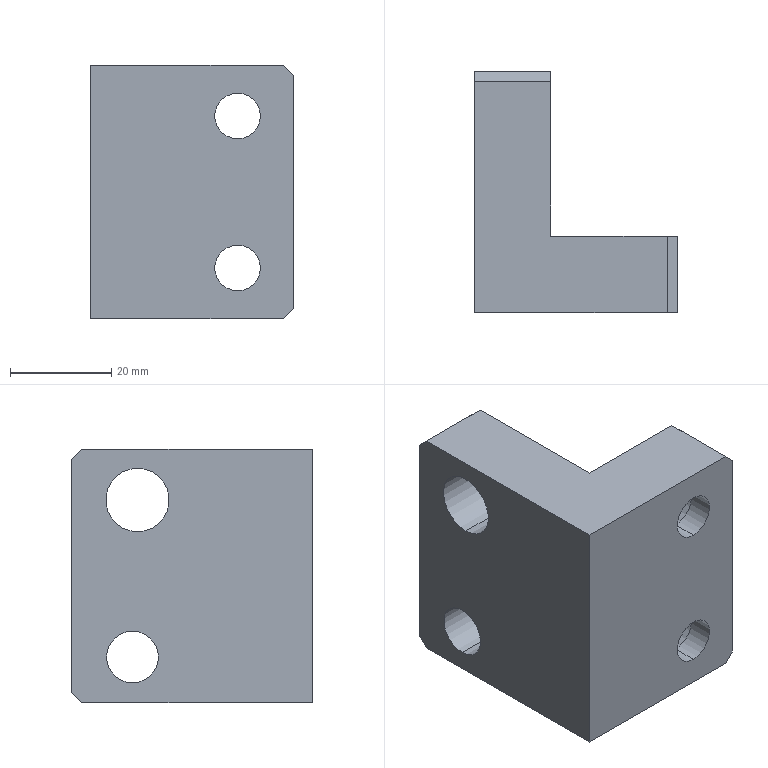Part | SolidWorks | features HoleWzd 3, Chamfer 1, Extrusion 1 | 1 solid | 26 faces | box 40 x 47.5 x 50 mm | volume 47018 mm3 | plane 14 | cylinder 12 | commonest cylinder face diameters 9 x4 15 x4 10.2 x2 12.5 x2
STEP:
#1=CARTESIAN_POINT('',(-40.82,7.906,14.1));
#2=VERTEX_POINT('',#1);
#3=CARTESIAN_POINT('',(-40.82,7.906,3.9));
#4=VERTEX_POINT('',#3);
#5=CARTESIAN_POINT('',(-40.82,7.906,9.));
#6=DIRECTION('',(1.,0.,0.));
#7=DIRECTION('',(0.,0.,-1.));
#8=AXIS2_PLACEMENT_3D('',#5,#6,#7);
#9=CIRCLE('',#8,5.1);
#10=EDGE_CURVE('',#2,#4,#9,.T.);
#11=ORIENTED_EDGE('',*,*,#10,.F.);
#12=CARTESIAN_POINT('',(-25.82,7.906,14.1));
#13=VERTEX_POINT('',#12);
#14=CARTESIAN_POINT('',(-25.82,7.906,14.1));
#15=DIRECTION('',(1.,0.,0.));
#16=VECTOR('',#15,1000.);
#17=LINE('',#14,#16);
#18=EDGE_CURVE('',#2,#13,#17,.T.);
#19=ORIENTED_EDGE('',*,*,#18,.T.);
#20=CARTESIAN_POINT('',(-25.82,7.906,3.9));
#21=VERTEX_POINT('',#20);
#22=CARTESIAN_POINT('',(-25.82,7.906,9.));
#23=DIRECTION('',(1.,0.,0.));
#24=DIRECTION('',(0.,0.,-1.));
#25=AXIS2_PLACEMENT_3D('',#22,#23,#24);
#26=CIRCLE('',#25,5.1);
#27=EDGE_CURVE('',#13,#21,#26,.T.);
#28=ORIENTED_EDGE('',*,*,#27,.T.);
#29=CARTESIAN_POINT('',(-25.82,7.906,3.9));
#30=DIRECTION('',(1.,0.,0.));
#31=VECTOR('',#30,1000.);
#32=LINE('',#29,#31);
#33=EDGE_CURVE('',#4,#21,#32,.T.);
#34=ORIENTED_EDGE('',*,*,#33,.F.);
#35=EDGE_LOOP('',(#11,#19,#28,#34));
#36=FACE_OUTER_BOUND('',#35,.T.);
#37=CARTESIAN_POINT('',(-25.82,7.906,9.));
#38=DIRECTION('',(1.,0.,0.));
#39=DIRECTION('',(0.,0.,-1.));
#40=AXIS2_PLACEMENT_3D('',#37,#38,#39);
#41=CYLINDRICAL_SURFACE('',#40,5.1);
#42=ADVANCED_FACE('',(#36),#41,.F.);
#43=CARTESIAN_POINT('',(-40.82,6.906,46.25));
#44=VERTEX_POINT('',#43);
#45=CARTESIAN_POINT('',(-40.82,6.906,33.75));
#46=VERTEX_POINT('',#45);
#47=CARTESIAN_POINT('',(-40.82,6.906,40.));
#48=DIRECTION('',(1.,0.,0.));
#49=DIRECTION('',(0.,0.,-1.));
#50=AXIS2_PLACEMENT_3D('',#47,#48,#49);
#51=CIRCLE('',#50,6.25);
#52=EDGE_CURVE('',#44,#46,#51,.T.);
#53=ORIENTED_EDGE('',*,*,#52,.F.);
#54=CARTESIAN_POINT('',(-25.82,6.906,46.25));
#55=VERTEX_POINT('',#54);
#56=CARTESIAN_POINT('',(-25.82,6.906,46.25));
#57=DIRECTION('',(1.,0.,0.));
#58=VECTOR('',#57,1000.);
#59=LINE('',#56,#58);
#60=EDGE_CURVE('',#44,#55,#59,.T.);
#61=ORIENTED_EDGE('',*,*,#60,.T.);
#62=CARTESIAN_POINT('',(-25.82,6.906,33.75));
#63=VERTEX_POINT('',#62);
#64=CARTESIAN_POINT('',(-25.82,6.906,40.));
#65=DIRECTION('',(1.,0.,0.));
#66=DIRECTION('',(0.,0.,-1.));
#67=AXIS2_PLACEMENT_3D('',#64,#65,#66);
#68=CIRCLE('',#67,6.25);
#69=EDGE_CURVE('',#55,#63,#68,.T.);
#70=ORIENTED_EDGE('',*,*,#69,.T.);
#71=CARTESIAN_POINT('',(-25.82,6.906,33.75));
#72=DIRECTION('',(1.,0.,0.));
#73=VECTOR('',#72,1000.);
#74=LINE('',#71,#73);
#75=EDGE_CURVE('',#46,#63,#74,.T.);
#76=ORIENTED_EDGE('',*,*,#75,.F.);
#77=EDGE_LOOP('',(#53,#61,#70,#76));
#78=FACE_OUTER_BOUND('',#77,.T.);
#79=CARTESIAN_POINT('',(-25.82,6.906,40.));
#80=DIRECTION('',(1.,0.,0.));
#81=DIRECTION('',(0.,0.,-1.));
#82=AXIS2_PLACEMENT_3D('',#79,#80,#81);
#83=CYLINDRICAL_SURFACE('',#82,6.25);
#84=ADVANCED_FACE('',(#78),#83,.F.);
#85=CARTESIAN_POINT('',(-11.82,-22.594,2.5));
#86=VERTEX_POINT('',#85);
#87=CARTESIAN_POINT('',(-11.82,-22.594,17.5));
#88=VERTEX_POINT('',#87);
#89=CARTESIAN_POINT('',(-11.82,-22.594,10.));
#90=DIRECTION('',(0.,1.,0.));
#91=DIRECTION('',(0.,0.,1.));
#92=AXIS2_PLACEMENT_3D('',#89,#90,#91);
#93=CIRCLE('',#92,7.5);
#94=EDGE_CURVE('',#86,#88,#93,.T.);
#95=ORIENTED_EDGE('',*,*,#94,.F.);
#96=CARTESIAN_POINT('',(-11.82,-12.594,2.5));
#97=VERTEX_POINT('',#96);
#98=CARTESIAN_POINT('',(-11.82,-12.594,2.5));
#99=DIRECTION('',(0.,1.,0.));
#100=VECTOR('',#99,1000.);
#101=LINE('',#98,#100);
#102=EDGE_CURVE('',#86,#97,#101,.T.);
#103=ORIENTED_EDGE('',*,*,#102,.T.);
#104=CARTESIAN_POINT('',(-11.82,-12.594,17.5));
#105=VERTEX_POINT('',#104);
#106=CARTESIAN_POINT('',(-11.82,-12.594,10.));
#107=DIRECTION('',(0.,1.,0.));
#108=DIRECTION('',(0.,0.,1.));
#109=AXIS2_PLACEMENT_3D('',#106,#107,#108);
#110=CIRCLE('',#109,7.5);
#111=EDGE_CURVE('',#97,#105,#110,.T.);
#112=ORIENTED_EDGE('',*,*,#111,.T.);
#113=CARTESIAN_POINT('',(-11.82,-12.594,17.5));
#114=DIRECTION('',(0.,1.,0.));
#115=VECTOR('',#114,1000.);
#116=LINE('',#113,#115);
#117=EDGE_CURVE('',#88,#105,#116,.T.);
#118=ORIENTED_EDGE('',*,*,#117,.F.);
#119=EDGE_LOOP('',(#95,#103,#112,#118));
#120=FACE_OUTER_BOUND('',#119,.T.);
#121=CARTESIAN_POINT('',(-11.82,-12.594,10.));
#122=DIRECTION('',(0.,1.,0.));
#123=DIRECTION('',(0.,0.,1.));
#124=AXIS2_PLACEMENT_3D('',#121,#122,#123);
#125=CYLINDRICAL_SURFACE('',#124,7.5);
#126=ADVANCED_FACE('',(#120),#125,.F.);
#127=CARTESIAN_POINT('',(-11.82,-27.594,5.5));
#128=VERTEX_POINT('',#127);
#129=CARTESIAN_POINT('',(-11.82,-27.594,14.5));
#130=VERTEX_POINT('',#129);
#131=CARTESIAN_POINT('',(-11.82,-27.594,10.));
#132=DIRECTION('',(0.,1.,0.));
#133=DIRECTION('',(0.,0.,1.));
#134=AXIS2_PLACEMENT_3D('',#131,#132,#133);
#135=CIRCLE('',#134,4.5);
#136=EDGE_CURVE('',#128,#130,#135,.T.);
#137=ORIENTED_EDGE('',*,*,#136,.F.);
#138=CARTESIAN_POINT('',(-11.82,-22.594,5.5));
#139=VERTEX_POINT('',#138);
#140=CARTESIAN_POINT('',(-11.82,-12.594,5.5));
#141=DIRECTION('',(0.,1.,0.));
#142=VECTOR('',#141,1000.);
#143=LINE('',#140,#142);
#144=EDGE_CURVE('',#128,#139,#143,.T.);
#145=ORIENTED_EDGE('',*,*,#144,.T.);
#146=CARTESIAN_POINT('',(-11.82,-22.594,14.5));
#147=VERTEX_POINT('',#146);
#148=CARTESIAN_POINT('',(-11.82,-22.594,10.));
#149=DIRECTION('',(0.,1.,0.));
#150=DIRECTION('',(0.,0.,1.));
#151=AXIS2_PLACEMENT_3D('',#148,#149,#150);
#152=CIRCLE('',#151,4.5);
#153=EDGE_CURVE('',#139,#147,#152,.T.);
#154=ORIENTED_EDGE('',*,*,#153,.T.);
#155=CARTESIAN_POINT('',(-11.82,-12.594,14.5));
#156=DIRECTION('',(0.,1.,0.));
#157=VECTOR('',#156,1000.);
#158=LINE('',#155,#157);
#159=EDGE_CURVE('',#130,#147,#158,.T.);
#160=ORIENTED_EDGE('',*,*,#159,.F.);
#161=EDGE_LOOP('',(#137,#145,#154,#160));
#162=FACE_OUTER_BOUND('',#161,.T.);
#163=CARTESIAN_POINT('',(-11.82,-12.594,10.));
#164=DIRECTION('',(0.,1.,0.));
#165=DIRECTION('',(0.,0.,1.));
#166=AXIS2_PLACEMENT_3D('',#163,#164,#165);
#167=CYLINDRICAL_SURFACE('',#166,4.5);
#168=ADVANCED_FACE('',(#162),#167,.F.);
#169=CARTESIAN_POINT('',(-11.82,-22.594,32.5));
#170=VERTEX_POINT('',#169);
#171=CARTESIAN_POINT('',(-11.82,-22.594,47.5));
#172=VERTEX_POINT('',#171);
#173=CARTESIAN_POINT('',(-11.82,-22.594,40.));
#174=DIRECTION('',(0.,1.,0.));
#175=DIRECTION('',(0.,0.,1.));
#176=AXIS2_PLACEMENT_3D('',#173,#174,#175);
#177=CIRCLE('',#176,7.5);
#178=EDGE_CURVE('',#170,#172,#177,.T.);
#179=ORIENTED_EDGE('',*,*,#178,.F.);
#180=CARTESIAN_POINT('',(-11.82,-12.594,32.5));
#181=VERTEX_POINT('',#180);
#182=CARTESIAN_POINT('',(-11.82,-12.594,32.5));
#183=DIRECTION('',(0.,1.,0.));
#184=VECTOR('',#183,1000.);
#185=LINE('',#182,#184);
#186=EDGE_CURVE('',#170,#181,#185,.T.);
#187=ORIENTED_EDGE('',*,*,#186,.T.);
#188=CARTESIAN_POINT('',(-11.82,-12.594,47.5));
#189=VERTEX_POINT('',#188);
#190=CARTESIAN_POINT('',(-11.82,-12.594,40.));
#191=DIRECTION('',(0.,1.,0.));
#192=DIRECTION('',(0.,0.,1.));
#193=AXIS2_PLACEMENT_3D('',#190,#191,#192);
#194=CIRCLE('',#193,7.5);
#195=EDGE_CURVE('',#181,#189,#194,.T.);
#196=ORIENTED_EDGE('',*,*,#195,.T.);
#197=CARTESIAN_POINT('',(-11.82,-12.594,47.5));
#198=DIRECTION('',(0.,1.,0.));
#199=VECTOR('',#198,1000.);
#200=LINE('',#197,#199);
#201=EDGE_CURVE('',#172,#189,#200,.T.);
#202=ORIENTED_EDGE('',*,*,#201,.F.);
#203=EDGE_LOOP('',(#179,#187,#196,#202));
#204=FACE_OUTER_BOUND('',#203,.T.);
#205=CARTESIAN_POINT('',(-11.82,-12.594,40.));
#206=DIRECTION('',(0.,1.,0.));
#207=DIRECTION('',(0.,0.,1.));
#208=AXIS2_PLACEMENT_3D('',#205,#206,#207);
#209=CYLINDRICAL_SURFACE('',#208,7.5);
#210=ADVANCED_FACE('',(#204),#209,.F.);
#211=CARTESIAN_POINT('',(-11.82,-27.594,35.5));
#212=VERTEX_POINT('',#211);
#213=CARTESIAN_POINT('',(-11.82,-27.594,44.5));
#214=VERTEX_POINT('',#213);
#215=CARTESIAN_POINT('',(-11.82,-27.594,40.));
#216=DIRECTION('',(0.,1.,0.));
#217=DIRECTION('',(0.,0.,1.));
#218=AXIS2_PLACEMENT_3D('',#215,#216,#217);
#219=CIRCLE('',#218,4.5);
#220=EDGE_CURVE('',#212,#214,#219,.T.);
#221=ORIENTED_EDGE('',*,*,#220,.F.);
#222=CARTESIAN_POINT('',(-11.82,-22.594,35.5));
#223=VERTEX_POINT('',#222);
#224=CARTESIAN_POINT('',(-11.82,-12.594,35.5));
#225=DIRECTION('',(0.,1.,0.));
#226=VECTOR('',#225,1000.);
#227=LINE('',#224,#226);
#228=EDGE_CURVE('',#212,#223,#227,.T.);
#229=ORIENTED_EDGE('',*,*,#228,.T.);
#230=CARTESIAN_POINT('',(-11.82,-22.594,44.5));
#231=VERTEX_POINT('',#230);
#232=CARTESIAN_POINT('',(-11.82,-22.594,40.));
#233=DIRECTION('',(0.,1.,0.));
#234=DIRECTION('',(0.,0.,1.));
#235=AXIS2_PLACEMENT_3D('',#232,#233,#234);
#236=CIRCLE('',#235,4.5);
#237=EDGE_CURVE('',#223,#231,#236,.T.);
#238=ORIENTED_EDGE('',*,*,#237,.T.);
#239=CARTESIAN_POINT('',(-11.82,-12.594,44.5));
#240=DIRECTION('',(0.,1.,0.));
#241=VECTOR('',#240,1000.);
#242=LINE('',#239,#241);
#243=EDGE_CURVE('',#214,#231,#242,.T.);
#244=ORIENTED_EDGE('',*,*,#243,.F.);
#245=EDGE_LOOP('',(#221,#229,#238,#244));
#246=FACE_OUTER_BOUND('',#245,.T.);
#247=CARTESIAN_POINT('',(-11.82,-12.594,40.));
#248=DIRECTION('',(0.,1.,0.));
#249=DIRECTION('',(0.,0.,1.));
#250=AXIS2_PLACEMENT_3D('',#247,#248,#249);
#251=CYLINDRICAL_SURFACE('',#250,4.5);
#252=ADVANCED_FACE('',(#246),#251,.F.);
#253=CARTESIAN_POINT('',(-25.82,19.906,48.));
#254=VERTEX_POINT('',#253);
#255=CARTESIAN_POINT('',(-25.82,19.906,2.));
#256=VERTEX_POINT('',#255);
#257=CARTESIAN_POINT('',(-25.82,19.906,50.));
#258=DIRECTION('',(0.,0.,-1.));
#259=VECTOR('',#258,1000.);
#260=LINE('',#257,#259);
#261=EDGE_CURVE('',#254,#256,#260,.T.);
#262=ORIENTED_EDGE('',*,*,#261,.T.);
#263=CARTESIAN_POINT('',(-40.82,19.906,2.));
#264=VERTEX_POINT('',#263);
#265=CARTESIAN_POINT('',(-25.82,19.906,2.));
#266=DIRECTION('',(-1.,0.,0.));
#267=VECTOR('',#266,1000.);
#268=LINE('',#265,#267);
#269=EDGE_CURVE('',#256,#264,#268,.T.);
#270=ORIENTED_EDGE('',*,*,#269,.T.);
#271=CARTESIAN_POINT('',(-40.82,19.906,48.));
#272=VERTEX_POINT('',#271);
#273=CARTESIAN_POINT('',(-40.82,19.906,50.));
#274=DIRECTION('',(0.,0.,-1.));
#275=VECTOR('',#274,1000.);
#276=LINE('',#273,#275);
#277=EDGE_CURVE('',#272,#264,#276,.T.);
#278=ORIENTED_EDGE('',*,*,#277,.F.);
#279=CARTESIAN_POINT('',(-25.82,19.906,48.));
#280=DIRECTION('',(1.,0.,0.));
#281=VECTOR('',#280,1000.);
#282=LINE('',#279,#281);
#283=EDGE_CURVE('',#272,#254,#282,.T.);
#284=ORIENTED_EDGE('',*,*,#283,.T.);
#285=EDGE_LOOP('',(#262,#270,#278,#284));
#286=FACE_OUTER_BOUND('',#285,.T.);
#287=CARTESIAN_POINT('',(-25.82,19.906,50.));
#288=DIRECTION('',(0.,-1.,0.));
#289=DIRECTION('',(1.,0.,0.));
#290=AXIS2_PLACEMENT_3D('',#287,#288,#289);
#291=PLANE('',#290);
#292=ADVANCED_FACE('',(#286),#291,.F.);
#293=CARTESIAN_POINT('',(-40.82,7.906,9.));
#294=DIRECTION('',(1.,0.,0.));
#295=DIRECTION('',(0.,0.,-1.));
#296=AXIS2_PLACEMENT_3D('',#293,#294,#295);
#297=CIRCLE('',#296,5.1);
#298=EDGE_CURVE('',#4,#2,#297,.T.);
#299=ORIENTED_EDGE('',*,*,#298,.T.);
#300=ORIENTED_EDGE('',*,*,#10,.T.);
#301=EDGE_LOOP('',(#299,#300));
#302=FACE_BOUND('',#301,.T.);
#303=CARTESIAN_POINT('',(-40.82,6.906,40.));
#304=DIRECTION('',(1.,0.,0.));
#305=DIRECTION('',(0.,0.,-1.));
#306=AXIS2_PLACEMENT_3D('',#303,#304,#305);
#307=CIRCLE('',#306,6.25);
#308=EDGE_CURVE('',#46,#44,#307,.T.);
#309=ORIENTED_EDGE('',*,*,#308,.T.);
#310=ORIENTED_EDGE('',*,*,#52,.T.);
#311=EDGE_LOOP('',(#309,#310));
#312=FACE_BOUND('',#311,.T.);
#313=ORIENTED_EDGE('',*,*,#277,.T.);
#314=CARTESIAN_POINT('',(-40.82,17.906,0.));
#315=VERTEX_POINT('',#314);
#316=CARTESIAN_POINT('',(-40.82,19.906,2.));
#317=DIRECTION('',(0.,-0.7071,-0.7071));
#318=VECTOR('',#317,1000.);
#319=LINE('',#316,#318);
#320=EDGE_CURVE('',#264,#315,#319,.T.);
#321=ORIENTED_EDGE('',*,*,#320,.T.);
#322=CARTESIAN_POINT('',(-40.82,-27.594,0.));
#323=VERTEX_POINT('',#322);
#324=CARTESIAN_POINT('',(-40.82,19.906,0.));
#325=DIRECTION('',(0.,-1.,0.));
#326=VECTOR('',#325,1000.);
#327=LINE('',#324,#326);
#328=EDGE_CURVE('',#315,#323,#327,.T.);
#329=ORIENTED_EDGE('',*,*,#328,.T.);
#330=CARTESIAN_POINT('',(-40.82,-27.594,50.));
#331=VERTEX_POINT('',#330);
#332=CARTESIAN_POINT('',(-40.82,-27.594,50.));
#333=DIRECTION('',(0.,0.,-1.));
#334=VECTOR('',#333,1000.);
#335=LINE('',#332,#334);
#336=EDGE_CURVE('',#331,#323,#335,.T.);
#337=ORIENTED_EDGE('',*,*,#336,.F.);
#338=CARTESIAN_POINT('',(-40.82,17.906,50.));
#339=VERTEX_POINT('',#338);
#340=CARTESIAN_POINT('',(-40.82,19.906,50.));
#341=DIRECTION('',(0.,-1.,0.));
#342=VECTOR('',#341,1000.);
#343=LINE('',#340,#342);
#344=EDGE_CURVE('',#339,#331,#343,.T.);
#345=ORIENTED_EDGE('',*,*,#344,.F.);
#346=CARTESIAN_POINT('',(-40.82,17.906,50.));
#347=DIRECTION('',(0.,0.7071,-0.7071));
#348=VECTOR('',#347,1000.);
#349=LINE('',#346,#348);
#350=EDGE_CURVE('',#339,#272,#349,.T.);
#351=ORIENTED_EDGE('',*,*,#350,.T.);
#352=EDGE_LOOP('',(#313,#321,#329,#337,#345,#351));
#353=FACE_OUTER_BOUND('',#352,.T.);
#354=CARTESIAN_POINT('',(-40.82,19.906,50.));
#355=DIRECTION('',(1.,0.,0.));
#356=DIRECTION('',(0.,1.,0.));
#357=AXIS2_PLACEMENT_3D('',#354,#355,#356);
#358=PLANE('',#357);
#359=ADVANCED_FACE('',(#302,#312,#353),#358,.F.);
#360=CARTESIAN_POINT('',(-11.82,-27.594,10.));
#361=DIRECTION('',(0.,1.,0.));
#362=DIRECTION('',(0.,0.,1.));
#363=AXIS2_PLACEMENT_3D('',#360,#361,#362);
#364=CIRCLE('',#363,4.5);
#365=EDGE_CURVE('',#130,#128,#364,.T.);
#366=ORIENTED_EDGE('',*,*,#365,.T.);
#367=ORIENTED_EDGE('',*,*,#136,.T.);
#368=EDGE_LOOP('',(#366,#367));
#369=FACE_BOUND('',#368,.T.);
#370=CARTESIAN_POINT('',(-11.82,-27.594,40.));
#371=DIRECTION('',(0.,1.,0.));
#372=DIRECTION('',(0.,0.,1.));
#373=AXIS2_PLACEMENT_3D('',#370,#371,#372);
#374=CIRCLE('',#373,4.5);
#375=EDGE_CURVE('',#214,#212,#374,.T.);
#376=ORIENTED_EDGE('',*,*,#375,.T.);
#377=ORIENTED_EDGE('',*,*,#220,.T.);
#378=EDGE_LOOP('',(#376,#377));
#379=FACE_BOUND('',#378,.T.);
#380=CARTESIAN_POINT('',(-2.82,-27.594,0.));
#381=VERTEX_POINT('',#380);
#382=CARTESIAN_POINT('',(-40.82,-27.594,0.));
#383=DIRECTION('',(1.,0.,0.));
#384=VECTOR('',#383,1000.);
#385=LINE('',#382,#384);
#386=EDGE_CURVE('',#323,#381,#385,.T.);
#387=ORIENTED_EDGE('',*,*,#386,.T.);
#388=CARTESIAN_POINT('',(-0.8198,-27.594,2.));
#389=VERTEX_POINT('',#388);
#390=CARTESIAN_POINT('',(-0.8198,-27.594,2.));
#391=DIRECTION('',(0.7071,0.,0.7071));
#392=VECTOR('',#391,1000.);
#393=LINE('',#390,#392);
#394=EDGE_CURVE('',#381,#389,#393,.T.);
#395=ORIENTED_EDGE('',*,*,#394,.T.);
#396=CARTESIAN_POINT('',(-0.8198,-27.594,48.));
#397=VERTEX_POINT('',#396);
#398=CARTESIAN_POINT('',(-0.8198,-27.594,50.));
#399=DIRECTION('',(0.,0.,-1.));
#400=VECTOR('',#399,1000.);
#401=LINE('',#398,#400);
#402=EDGE_CURVE('',#397,#389,#401,.T.);
#403=ORIENTED_EDGE('',*,*,#402,.F.);
#404=CARTESIAN_POINT('',(-2.82,-27.594,50.));
#405=VERTEX_POINT('',#404);
#406=CARTESIAN_POINT('',(-2.82,-27.594,50.));
#407=DIRECTION('',(-0.7071,0.,0.7071));
#408=VECTOR('',#407,1000.);
#409=LINE('',#406,#408);
#410=EDGE_CURVE('',#397,#405,#409,.T.);
#411=ORIENTED_EDGE('',*,*,#410,.T.);
#412=CARTESIAN_POINT('',(-40.82,-27.594,50.));
#413=DIRECTION('',(1.,0.,0.));
#414=VECTOR('',#413,1000.);
#415=LINE('',#412,#414);
#416=EDGE_CURVE('',#331,#405,#415,.T.);
#417=ORIENTED_EDGE('',*,*,#416,.F.);
#418=ORIENTED_EDGE('',*,*,#336,.T.);
#419=EDGE_LOOP('',(#387,#395,#403,#411,#417,#418));
#420=FACE_OUTER_BOUND('',#419,.T.);
#421=CARTESIAN_POINT('',(-40.82,-27.594,50.));
#422=DIRECTION('',(0.,1.,0.));
#423=DIRECTION('',(0.,0.,1.));
#424=AXIS2_PLACEMENT_3D('',#421,#422,#423);
#425=PLANE('',#424);
#426=ADVANCED_FACE('',(#369,#379,#420),#425,.F.);
#427=ORIENTED_EDGE('',*,*,#402,.T.);
#428=CARTESIAN_POINT('',(-0.8198,-12.594,2.));
#429=VERTEX_POINT('',#428);
#430=CARTESIAN_POINT('',(-0.8198,-27.594,2.));
#431=DIRECTION('',(0.,1.,0.));
#432=VECTOR('',#431,1000.);
#433=LINE('',#430,#432);
#434=EDGE_CURVE('',#389,#429,#433,.T.);
#435=ORIENTED_EDGE('',*,*,#434,.T.);
#436=CARTESIAN_POINT('',(-0.8198,-12.594,48.));
#437=VERTEX_POINT('',#436);
#438=CARTESIAN_POINT('',(-0.8198,-12.594,50.));
#439=DIRECTION('',(0.,0.,-1.));
#440=VECTOR('',#439,1000.);
#441=LINE('',#438,#440);
#442=EDGE_CURVE('',#437,#429,#441,.T.);
#443=ORIENTED_EDGE('',*,*,#442,.F.);
#444=CARTESIAN_POINT('',(-0.8198,-27.594,48.));
#445=DIRECTION('',(0.,-1.,0.));
#446=VECTOR('',#445,1000.);
#447=LINE('',#444,#446);
#448=EDGE_CURVE('',#437,#397,#447,.T.);
#449=ORIENTED_EDGE('',*,*,#448,.T.);
#450=EDGE_LOOP('',(#427,#435,#443,#449));
#451=FACE_OUTER_BOUND('',#450,.T.);
#452=CARTESIAN_POINT('',(-0.8198,-27.594,50.));
#453=DIRECTION('',(-1.,0.,0.));
#454=DIRECTION('',(0.,0.,1.));
#455=AXIS2_PLACEMENT_3D('',#452,#453,#454);
#456=PLANE('',#455);
#457=ADVANCED_FACE('',(#451),#456,.F.);
#458=CARTESIAN_POINT('',(-11.82,-12.594,10.));
#459=DIRECTION('',(0.,1.,0.));
#460=DIRECTION('',(0.,0.,1.));
#461=AXIS2_PLACEMENT_3D('',#458,#459,#460);
#462=CIRCLE('',#461,7.5);
#463=EDGE_CURVE('',#105,#97,#462,.T.);
#464=ORIENTED_EDGE('',*,*,#463,.F.);
#465=ORIENTED_EDGE('',*,*,#111,.F.);
#466=EDGE_LOOP('',(#464,#465));
#467=FACE_BOUND('',#466,.T.);
#468=CARTESIAN_POINT('',(-11.82,-12.594,40.));
#469=DIRECTION('',(0.,1.,0.));
#470=DIRECTION('',(0.,0.,1.));
#471=AXIS2_PLACEMENT_3D('',#468,#469,#470);
#472=CIRCLE('',#471,7.5);
#473=EDGE_CURVE('',#189,#181,#472,.T.);
#474=ORIENTED_EDGE('',*,*,#473,.F.);
#475=ORIENTED_EDGE('',*,*,#195,.F.);
#476=EDGE_LOOP('',(#474,#475));
#477=FACE_BOUND('',#476,.T.);
#478=ORIENTED_EDGE('',*,*,#442,.T.);
#479=CARTESIAN_POINT('',(-2.82,-12.594,0.));
#480=VERTEX_POINT('',#479);
#481=CARTESIAN_POINT('',(-0.8198,-12.594,2.));
#482=DIRECTION('',(-0.7071,0.,-0.7071));
#483=VECTOR('',#482,1000.);
#484=LINE('',#481,#483);
#485=EDGE_CURVE('',#429,#480,#484,.T.);
#486=ORIENTED_EDGE('',*,*,#485,.T.);
#487=CARTESIAN_POINT('',(-25.82,-12.594,0.));
#488=VERTEX_POINT('',#487);
#489=CARTESIAN_POINT('',(-0.8198,-12.594,0.));
#490=DIRECTION('',(-1.,0.,0.));
#491=VECTOR('',#490,1000.);
#492=LINE('',#489,#491);
#493=EDGE_CURVE('',#480,#488,#492,.T.);
#494=ORIENTED_EDGE('',*,*,#493,.T.);
#495=CARTESIAN_POINT('',(-25.82,-12.594,50.));
#496=VERTEX_POINT('',#495);
#497=CARTESIAN_POINT('',(-25.82,-12.594,50.));
#498=DIRECTION('',(0.,0.,-1.));
#499=VECTOR('',#498,1000.);
#500=LINE('',#497,#499);
#501=EDGE_CURVE('',#496,#488,#500,.T.);
#502=ORIENTED_EDGE('',*,*,#501,.F.);
#503=CARTESIAN_POINT('',(-2.82,-12.594,50.));
#504=VERTEX_POINT('',#503);
#505=CARTESIAN_POINT('',(-0.8198,-12.594,50.));
#506=DIRECTION('',(-1.,0.,0.));
#507=VECTOR('',#506,1000.);
#508=LINE('',#505,#507);
#509=EDGE_CURVE('',#504,#496,#508,.T.);
#510=ORIENTED_EDGE('',*,*,#509,.F.);
#511=CARTESIAN_POINT('',(-2.82,-12.594,50.));
#512=DIRECTION('',(0.7071,0.,-0.7071));
#513=VECTOR('',#512,1000.);
#514=LINE('',#511,#513);
#515=EDGE_CURVE('',#504,#437,#514,.T.);
#516=ORIENTED_EDGE('',*,*,#515,.T.);
#517=EDGE_LOOP('',(#478,#486,#494,#502,#510,#516));
#518=FACE_OUTER_BOUND('',#517,.T.);
#519=CARTESIAN_POINT('',(-0.8198,-12.594,50.));
#520=DIRECTION('',(0.,-1.,0.));
#521=DIRECTION('',(1.,0.,0.));
#522=AXIS2_PLACEMENT_3D('',#519,#520,#521);
#523=PLANE('',#522);
#524=ADVANCED_FACE('',(#467,#477,#518),#523,.F.);
#525=CARTESIAN_POINT('',(-25.82,7.906,9.));
#526=DIRECTION('',(1.,0.,0.));
#527=DIRECTION('',(0.,0.,-1.));
#528=AXIS2_PLACEMENT_3D('',#525,#526,#527);
#529=CIRCLE('',#528,5.1);
#530=EDGE_CURVE('',#21,#13,#529,.T.);
#531=ORIENTED_EDGE('',*,*,#530,.F.);
#532=ORIENTED_EDGE('',*,*,#27,.F.);
#533=EDGE_LOOP('',(#531,#532));
#534=FACE_BOUND('',#533,.T.);
#535=CARTESIAN_POINT('',(-25.82,6.906,40.));
#536=DIRECTION('',(1.,0.,0.));
#537=DIRECTION('',(0.,0.,-1.));
#538=AXIS2_PLACEMENT_3D('',#535,#536,#537);
#539=CIRCLE('',#538,6.25);
#540=EDGE_CURVE('',#63,#55,#539,.T.);
#541=ORIENTED_EDGE('',*,*,#540,.F.);
#542=ORIENTED_EDGE('',*,*,#69,.F.);
#543=EDGE_LOOP('',(#541,#542));
#544=FACE_BOUND('',#543,.T.);
#545=CARTESIAN_POINT('',(-25.82,17.906,0.));
#546=VERTEX_POINT('',#545);
#547=CARTESIAN_POINT('',(-25.82,-12.594,0.));
#548=DIRECTION('',(0.,1.,0.));
#549=VECTOR('',#548,1000.);
#550=LINE('',#547,#549);
#551=EDGE_CURVE('',#488,#546,#550,.T.);
#552=ORIENTED_EDGE('',*,*,#551,.T.);
#553=CARTESIAN_POINT('',(-25.82,19.906,2.));
#554=DIRECTION('',(0.,0.7071,0.7071));
#555=VECTOR('',#554,1000.);
#556=LINE('',#553,#555);
#557=EDGE_CURVE('',#546,#256,#556,.T.);
#558=ORIENTED_EDGE('',*,*,#557,.T.);
#559=ORIENTED_EDGE('',*,*,#261,.F.);
#560=CARTESIAN_POINT('',(-25.82,17.906,50.));
#561=VERTEX_POINT('',#560);
#562=CARTESIAN_POINT('',(-25.82,17.906,50.));
#563=DIRECTION('',(0.,-0.7071,0.7071));
#564=VECTOR('',#563,1000.);
#565=LINE('',#562,#564);
#566=EDGE_CURVE('',#254,#561,#565,.T.);
#567=ORIENTED_EDGE('',*,*,#566,.T.);
#568=CARTESIAN_POINT('',(-25.82,-12.594,50.));
#569=DIRECTION('',(0.,1.,0.));
#570=VECTOR('',#569,1000.);
#571=LINE('',#568,#570);
#572=EDGE_CURVE('',#496,#561,#571,.T.);
#573=ORIENTED_EDGE('',*,*,#572,.F.);
#574=ORIENTED_EDGE('',*,*,#501,.T.);
#575=EDGE_LOOP('',(#552,#558,#559,#567,#573,#574));
#576=FACE_OUTER_BOUND('',#575,.T.);
#577=CARTESIAN_POINT('',(-25.82,-12.594,50.));
#578=DIRECTION('',(-1.,0.,0.));
#579=DIRECTION('',(0.,-1.,0.));
#580=AXIS2_PLACEMENT_3D('',#577,#578,#579);
#581=PLANE('',#580);
#582=ADVANCED_FACE('',(#534,#544,#576),#581,.F.);
#583=ORIENTED_EDGE('',*,*,#416,.T.);
#584=CARTESIAN_POINT('',(-2.82,-12.594,50.));
#585=DIRECTION('',(0.,1.,0.));
#586=VECTOR('',#585,1000.);
#587=LINE('',#584,#586);
#588=EDGE_CURVE('',#405,#504,#587,.T.);
#589=ORIENTED_EDGE('',*,*,#588,.T.);
#590=ORIENTED_EDGE('',*,*,#509,.T.);
#591=ORIENTED_EDGE('',*,*,#572,.T.);
#592=CARTESIAN_POINT('',(-40.82,17.906,50.));
#593=DIRECTION('',(-1.,0.,0.));
#594=VECTOR('',#593,1000.);
#595=LINE('',#592,#594);
#596=EDGE_CURVE('',#561,#339,#595,.T.);
#597=ORIENTED_EDGE('',*,*,#596,.T.);
#598=ORIENTED_EDGE('',*,*,#344,.T.);
#599=EDGE_LOOP('',(#583,#589,#590,#591,#597,#598));
#600=FACE_OUTER_BOUND('',#599,.T.);
#601=CARTESIAN_POINT('',(0.,0.,50.));
#602=DIRECTION('',(0.,0.,1.));
#603=DIRECTION('',(1.,0.,0.));
#604=AXIS2_PLACEMENT_3D('',#601,#602,#603);
#605=PLANE('',#604);
#606=ADVANCED_FACE('',(#600),#605,.T.);
#607=ORIENTED_EDGE('',*,*,#493,.F.);
#608=CARTESIAN_POINT('',(-2.82,0.,0.));
#609=DIRECTION('',(0.,-1.,0.));
#610=VECTOR('',#609,1000.);
#611=LINE('',#608,#610);
#612=EDGE_CURVE('',#480,#381,#611,.T.);
#613=ORIENTED_EDGE('',*,*,#612,.T.);
#614=ORIENTED_EDGE('',*,*,#386,.F.);
#615=ORIENTED_EDGE('',*,*,#328,.F.);
#616=CARTESIAN_POINT('',(0.,17.906,0.));
#617=DIRECTION('',(1.,0.,0.));
#618=VECTOR('',#617,1000.);
#619=LINE('',#616,#618);
#620=EDGE_CURVE('',#315,#546,#619,.T.);
#621=ORIENTED_EDGE('',*,*,#620,.T.);
#622=ORIENTED_EDGE('',*,*,#551,.F.);
#623=EDGE_LOOP('',(#607,#613,#614,#615,#621,#622));
#624=FACE_OUTER_BOUND('',#623,.T.);
#625=CARTESIAN_POINT('',(0.,0.,0.));
#626=DIRECTION('',(0.,0.,1.));
#627=DIRECTION('',(1.,0.,0.));
#628=AXIS2_PLACEMENT_3D('',#625,#626,#627);
#629=PLANE('',#628);
#630=ADVANCED_FACE('',(#624),#629,.F.);
#631=ORIENTED_EDGE('',*,*,#394,.F.);
#632=ORIENTED_EDGE('',*,*,#612,.F.);
#633=ORIENTED_EDGE('',*,*,#485,.F.);
#634=ORIENTED_EDGE('',*,*,#434,.F.);
#635=EDGE_LOOP('',(#631,#632,#633,#634));
#636=FACE_OUTER_BOUND('',#635,.T.);
#637=CARTESIAN_POINT('',(-0.8198,-27.594,2.));
#638=DIRECTION('',(-0.7071,0.,0.7071));
#639=DIRECTION('',(0.,1.,0.));
#640=AXIS2_PLACEMENT_3D('',#637,#638,#639);
#641=PLANE('',#640);
#642=ADVANCED_FACE('',(#636),#641,.F.);
#643=ORIENTED_EDGE('',*,*,#410,.F.);
#644=ORIENTED_EDGE('',*,*,#448,.F.);
#645=ORIENTED_EDGE('',*,*,#515,.F.);
#646=ORIENTED_EDGE('',*,*,#588,.F.);
#647=EDGE_LOOP('',(#643,#644,#645,#646));
#648=FACE_OUTER_BOUND('',#647,.T.);
#649=CARTESIAN_POINT('',(-2.82,0.,50.));
#650=DIRECTION('',(0.7071,0.,0.7071));
#651=DIRECTION('',(0.,-1.,0.));
#652=AXIS2_PLACEMENT_3D('',#649,#650,#651);
#653=PLANE('',#652);
#654=ADVANCED_FACE('',(#648),#653,.T.);
#655=ORIENTED_EDGE('',*,*,#557,.F.);
#656=ORIENTED_EDGE('',*,*,#620,.F.);
#657=ORIENTED_EDGE('',*,*,#320,.F.);
#658=ORIENTED_EDGE('',*,*,#269,.F.);
#659=EDGE_LOOP('',(#655,#656,#657,#658));
#660=FACE_OUTER_BOUND('',#659,.T.);
#661=CARTESIAN_POINT('',(-25.82,19.906,2.));
#662=DIRECTION('',(0.,-0.7071,0.7071));
#663=DIRECTION('',(-1.,0.,0.));
#664=AXIS2_PLACEMENT_3D('',#661,#662,#663);
#665=PLANE('',#664);
#666=ADVANCED_FACE('',(#660),#665,.F.);
#667=ORIENTED_EDGE('',*,*,#566,.F.);
#668=ORIENTED_EDGE('',*,*,#283,.F.);
#669=ORIENTED_EDGE('',*,*,#350,.F.);
#670=ORIENTED_EDGE('',*,*,#596,.F.);
#671=EDGE_LOOP('',(#667,#668,#669,#670));
#672=FACE_OUTER_BOUND('',#671,.T.);
#673=CARTESIAN_POINT('',(0.,17.906,50.));
#674=DIRECTION('',(0.,0.7071,0.7071));
#675=DIRECTION('',(1.,0.,0.));
#676=AXIS2_PLACEMENT_3D('',#673,#674,#675);
#677=PLANE('',#676);
#678=ADVANCED_FACE('',(#672),#677,.T.);
#679=ORIENTED_EDGE('',*,*,#228,.F.);
#680=ORIENTED_EDGE('',*,*,#375,.F.);
#681=ORIENTED_EDGE('',*,*,#243,.T.);
#682=CARTESIAN_POINT('',(-11.82,-22.594,40.));
#683=DIRECTION('',(0.,1.,0.));
#684=DIRECTION('',(0.,0.,1.));
#685=AXIS2_PLACEMENT_3D('',#682,#683,#684);
#686=CIRCLE('',#685,4.5);
#687=EDGE_CURVE('',#231,#223,#686,.T.);
#688=ORIENTED_EDGE('',*,*,#687,.T.);
#689=EDGE_LOOP('',(#679,#680,#681,#688));
#690=FACE_OUTER_BOUND('',#689,.T.);
#691=CARTESIAN_POINT('',(-11.82,-12.594,40.));
#692=DIRECTION('',(0.,1.,0.));
#693=DIRECTION('',(0.,0.,1.));
#694=AXIS2_PLACEMENT_3D('',#691,#692,#693);
#695=CYLINDRICAL_SURFACE('',#694,4.5);
#696=ADVANCED_FACE('',(#690),#695,.F.);
#697=ORIENTED_EDGE('',*,*,#687,.F.);
#698=ORIENTED_EDGE('',*,*,#237,.F.);
#699=EDGE_LOOP('',(#697,#698));
#700=FACE_BOUND('',#699,.T.);
#701=CARTESIAN_POINT('',(-11.82,-22.594,40.));
#702=DIRECTION('',(0.,1.,0.));
#703=DIRECTION('',(0.,0.,1.));
#704=AXIS2_PLACEMENT_3D('',#701,#702,#703);
#705=CIRCLE('',#704,7.5);
#706=EDGE_CURVE('',#172,#170,#705,.T.);
#707=ORIENTED_EDGE('',*,*,#706,.T.);
#708=ORIENTED_EDGE('',*,*,#178,.T.);
#709=EDGE_LOOP('',(#707,#708));
#710=FACE_OUTER_BOUND('',#709,.T.);
#711=CARTESIAN_POINT('',(-7.32,-22.594,40.));
#712=DIRECTION('',(0.,-1.,0.));
#713=DIRECTION('',(0.,0.,-1.));
#714=AXIS2_PLACEMENT_3D('',#711,#712,#713);
#715=PLANE('',#714);
#716=ADVANCED_FACE('',(#700,#710),#715,.F.);
#717=ORIENTED_EDGE('',*,*,#186,.F.);
#718=ORIENTED_EDGE('',*,*,#706,.F.);
#719=ORIENTED_EDGE('',*,*,#201,.T.);
#720=ORIENTED_EDGE('',*,*,#473,.T.);
#721=EDGE_LOOP('',(#717,#718,#719,#720));
#722=FACE_OUTER_BOUND('',#721,.T.);
#723=CARTESIAN_POINT('',(-11.82,-12.594,40.));
#724=DIRECTION('',(0.,1.,0.));
#725=DIRECTION('',(0.,0.,1.));
#726=AXIS2_PLACEMENT_3D('',#723,#724,#725);
#727=CYLINDRICAL_SURFACE('',#726,7.5);
#728=ADVANCED_FACE('',(#722),#727,.F.);
#729=ORIENTED_EDGE('',*,*,#144,.F.);
#730=ORIENTED_EDGE('',*,*,#365,.F.);
#731=ORIENTED_EDGE('',*,*,#159,.T.);
#732=CARTESIAN_POINT('',(-11.82,-22.594,10.));
#733=DIRECTION('',(0.,1.,0.));
#734=DIRECTION('',(0.,0.,1.));
#735=AXIS2_PLACEMENT_3D('',#732,#733,#734);
#736=CIRCLE('',#735,4.5);
#737=EDGE_CURVE('',#147,#139,#736,.T.);
#738=ORIENTED_EDGE('',*,*,#737,.T.);
#739=EDGE_LOOP('',(#729,#730,#731,#738));
#740=FACE_OUTER_BOUND('',#739,.T.);
#741=CARTESIAN_POINT('',(-11.82,-12.594,10.));
#742=DIRECTION('',(0.,1.,0.));
#743=DIRECTION('',(0.,0.,1.));
#744=AXIS2_PLACEMENT_3D('',#741,#742,#743);
#745=CYLINDRICAL_SURFACE('',#744,4.5);
#746=ADVANCED_FACE('',(#740),#745,.F.);
#747=ORIENTED_EDGE('',*,*,#737,.F.);
#748=ORIENTED_EDGE('',*,*,#153,.F.);
#749=EDGE_LOOP('',(#747,#748));
#750=FACE_BOUND('',#749,.T.);
#751=CARTESIAN_POINT('',(-11.82,-22.594,10.));
#752=DIRECTION('',(0.,1.,0.));
#753=DIRECTION('',(0.,0.,1.));
#754=AXIS2_PLACEMENT_3D('',#751,#752,#753);
#755=CIRCLE('',#754,7.5);
#756=EDGE_CURVE('',#88,#86,#755,.T.);
#757=ORIENTED_EDGE('',*,*,#756,.T.);
#758=ORIENTED_EDGE('',*,*,#94,.T.);
#759=EDGE_LOOP('',(#757,#758));
#760=FACE_OUTER_BOUND('',#759,.T.);
#761=CARTESIAN_POINT('',(-7.32,-22.594,10.));
#762=DIRECTION('',(0.,-1.,0.));
#763=DIRECTION('',(0.,0.,-1.));
#764=AXIS2_PLACEMENT_3D('',#761,#762,#763);
#765=PLANE('',#764);
#766=ADVANCED_FACE('',(#750,#760),#765,.F.);
#767=ORIENTED_EDGE('',*,*,#102,.F.);
#768=ORIENTED_EDGE('',*,*,#756,.F.);
#769=ORIENTED_EDGE('',*,*,#117,.T.);
#770=ORIENTED_EDGE('',*,*,#463,.T.);
#771=EDGE_LOOP('',(#767,#768,#769,#770));
#772=FACE_OUTER_BOUND('',#771,.T.);
#773=CARTESIAN_POINT('',(-11.82,-12.594,10.));
#774=DIRECTION('',(0.,1.,0.));
#775=DIRECTION('',(0.,0.,1.));
#776=AXIS2_PLACEMENT_3D('',#773,#774,#775);
#777=CYLINDRICAL_SURFACE('',#776,7.5);
#778=ADVANCED_FACE('',(#772),#777,.F.);
#779=ORIENTED_EDGE('',*,*,#60,.F.);
#780=ORIENTED_EDGE('',*,*,#308,.F.);
#781=ORIENTED_EDGE('',*,*,#75,.T.);
#782=ORIENTED_EDGE('',*,*,#540,.T.);
#783=EDGE_LOOP('',(#779,#780,#781,#782));
#784=FACE_OUTER_BOUND('',#783,.T.);
#785=CARTESIAN_POINT('',(-25.82,6.906,40.));
#786=DIRECTION('',(1.,0.,0.));
#787=DIRECTION('',(0.,0.,-1.));
#788=AXIS2_PLACEMENT_3D('',#785,#786,#787);
#789=CYLINDRICAL_SURFACE('',#788,6.25);
#790=ADVANCED_FACE('',(#784),#789,.F.);
#791=ORIENTED_EDGE('',*,*,#18,.F.);
#792=ORIENTED_EDGE('',*,*,#298,.F.);
#793=ORIENTED_EDGE('',*,*,#33,.T.);
#794=ORIENTED_EDGE('',*,*,#530,.T.);
#795=EDGE_LOOP('',(#791,#792,#793,#794));
#796=FACE_OUTER_BOUND('',#795,.T.);
#797=CARTESIAN_POINT('',(-25.82,7.906,9.));
#798=DIRECTION('',(1.,0.,0.));
#799=DIRECTION('',(0.,0.,-1.));
#800=AXIS2_PLACEMENT_3D('',#797,#798,#799);
#801=CYLINDRICAL_SURFACE('',#800,5.1);
#802=ADVANCED_FACE('',(#796),#801,.F.);
#803=CLOSED_SHELL('',(#42,#84,#126,#168,#210,#252,#292,#359,#426,#457,#524,#582,#606,#630,#642,#654,#666,#678,#696,#716,#728,#746,#766,#778,#790,#802));
#804=MANIFOLD_SOLID_BREP('',#803);
#805=CARTESIAN_POINT('',(0.,0.,0.));
#806=DIRECTION('',(0.,0.,1.));
#807=DIRECTION('',(1.,0.,0.));
#808=AXIS2_PLACEMENT_3D('',#805,#806,#807);
#809=(LENGTH_UNIT()NAMED_UNIT(*)SI_UNIT(.MILLI.,.METRE.));
#810=UNCERTAINTY_MEASURE_WITH_UNIT(LENGTH_MEASURE(0.00001),#809,'','');
#811=(NAMED_UNIT(*)PLANE_ANGLE_UNIT()SI_UNIT($,.RADIAN.));
#812=(NAMED_UNIT(*)SI_UNIT($,.STERADIAN.)SOLID_ANGLE_UNIT());
#813=(GEOMETRIC_REPRESENTATION_CONTEXT(3)GLOBAL_UNCERTAINTY_ASSIGNED_CONTEXT((#810))GLOBAL_UNIT_ASSIGNED_CONTEXT((#809,#811,#812))REPRESENTATION_CONTEXT('',''));
#814=ADVANCED_BREP_SHAPE_REPRESENTATION('',(#804,#808),#813);